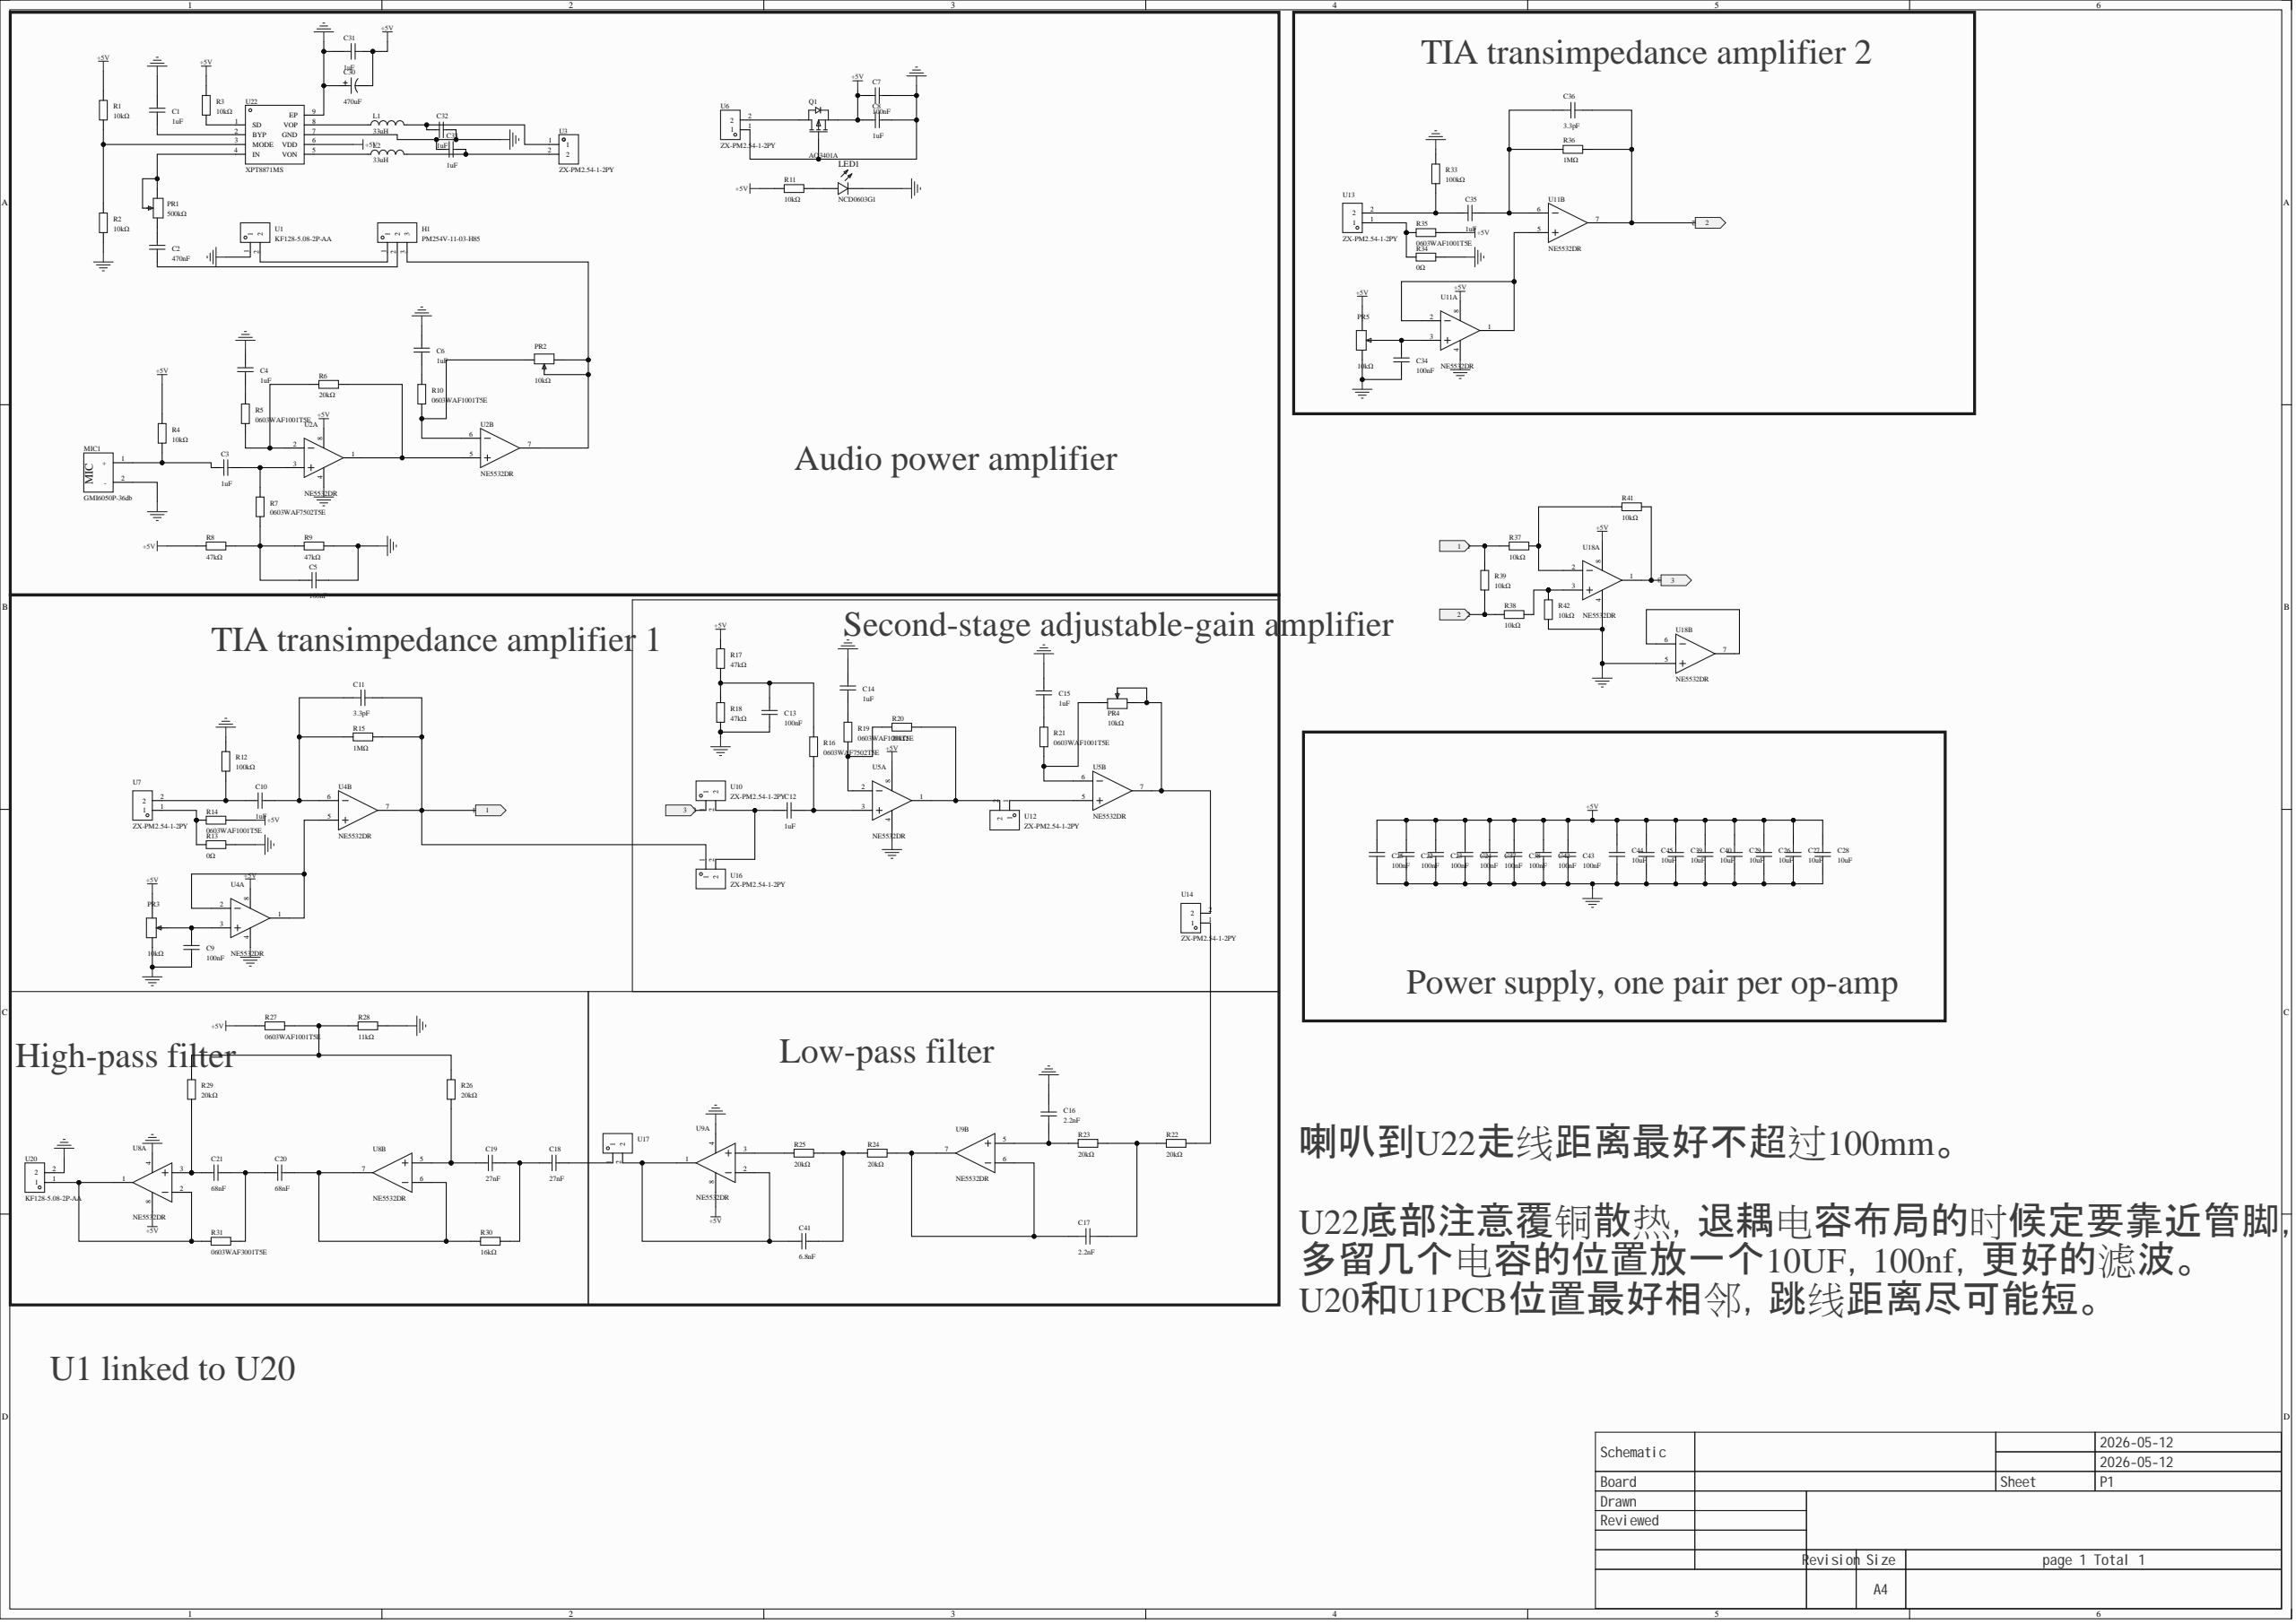Circuit board | Altium Designer | 115 parts | 65 nets
Bill of materials:
Comment,Description,Designator,Footprint,LibRef,Quantity
"1uF","Temperature coefficient: X5R; tolerance: ±10%; rated voltage: 50V; capacitance: 1uF;, Capacitance: 1uF; tolerance: ±10%; rated voltage: 50V; temperature coefficient: X5R;","C1, C3, C4, C6, C8, C10, C12, C14, C15, C31, C32, C33, C35","C0603","CL10A105KB8NNNC","13"
"470nF","Capacitance: 470nF; tolerance: ±10%; rated voltage: 16V; material (temperature coefficient): X7R;","C2","C0603","CC0603KRX7R7BB474","1"
"100nF","Capacitance: 100nF; tolerance: ±10%; rated voltage: 100V; material (temperature coefficient): X7R;","C5, C7, C9, C13, C22, C23, C24, C25, C34, C37, C38, C42, C43","C0805","CC0805KKX7R0BB104","13"
"3.3pF","Capacitance: 3.3pF; tolerance: ±0.1pF; rated voltage: 50V; material (temperature coefficient): NP0;","C11, C36","C0402","CC0402BRNPO9BN3R3","2"
"2.2nF","Temperature coefficient: X7R; capacitance: 2.2nF; tolerance: ±10%; rated voltage: 50V;","C16, C17","C0805","TCC0805X7R222K500DTS","2"
"27nF","Capacitance: 27nF; tolerance: ±10%; rated voltage: 50V; material (temperature coefficient): X7R;","C18, C19","C0603","CC0603KRX7R9BB273","2"
"68nF","Temperature coefficient: X7R; tolerance: ±10%; capacitance: 68nF; rated voltage: 50V;","C20, C21","C0603","CL10B683KB8NNNC","2"
"10uF","Capacitance: 10uF; tolerance: ±20%; rated voltage: 25V; temperature coefficient: X5R;","C26, C27, C28, C29, C39, C40, C44, C45","C0603","CL10A106MA8NRNC","8"
"470uF","Capacitance: 470uF; tolerance: ±20%; rated voltage: 35V;","C30","CAP-TH_BD10.0-P5.00-D1.0-FD","35YXJ470M10x16","1"
"6.8nF","Capacitance: 6.8nF; tolerance: ±10%; rated voltage: 50V; material (temperature coefficient): X7R;","C41","C0603","CC0603KRX7R9BB682","1"
"PM254V-11-03-H85","插孔结构:1x3P;间距:2.54mm;行距:-;圆孔/方孔:方孔;安装方式:直插;排数:单排;总孔位数:3P;额定电流:3A;插孔方向:顶部;塑高:8.5mm;触头材质:黄铜;触头镀层:-;工作温度:-40℃~+105℃;","H1","HDR-TH_3P-P2.54-V-F","PM254V-11-03-H85","1"
"33uH","Inductance: 33uH; tolerance: ±20%; rated current: 2A; DC resistance (DCR): 270mΩ;","L1, L2","IND-SMD_L7.3-W6.6","MHCI06030-330M-R8","2"
"NCD0603G1","Emitted color: emerald green;","LED1","LED0603-RD","NCD0603G1","1"
"GMI6050P-36db","","MIC1","MIC-TH_BD6.0-P1.90-D0.4-L-FD_GMI6050P-2CXXDB","GMI6050P-36db","1"
"500kΩ","Resistance: 500kΩ; tolerance: ±10%; temperature coefficient: ±100ppm/?;","PR1","RES-ADJ-TH_3296W","3296W-1-504LF","1"
"10kΩ","Resistance: 10kΩ; tolerance: ±10%; temperature coefficient: ±100ppm/?;","PR2, PR3, PR4, PR5","RES-ADJ-TH_3296W","3296W-1-103LF","4"
"AO3401A","","Q1","SOT-23_L2.9-W1.3-P1.90-LS2.4-BR","AO3401A_C15127","1"
"10kΩ","","R1, R2, R3, R4, R11, R37, R38, R39, R41, R42","R0603","0603WAF1002T5E","10"
"0603WAF1001T5E","","R5, R10, R14, R19, R21, R27, R35","R0603","0603WAF1001T5E","7"
"20kΩ","","R6, R20, R22, R23, R24, R25, R26, R29","R0603","0603WAF2002T5E","8"
"0603WAF7502T5E","","R7, R16","R0603","0603WAF7502T5E","2"
"47kΩ","","R8, R9, R17, R18","R0603","0603WAF4702T5E","4"
"100kΩ","","R12, R33","R0603","0603WAF1003T5E","2"
"0Ω","","R13, R34","R0603","0603WAF0000T5E","2"
"1MΩ","","R15, R36","R0603","0603WAF1004T5E","2"
"11kΩ","","R28","R0603","0603WAF1102T5E","1"
"16kΩ","","R30","R0603","0603WAF1602T5E","1"
"0603WAF3001T5E","","R31","R0603","0603WAF3001T5E","1"
"KF128-5.08-2P-AA","结构:1x2P;间距:5.08mm;颜色:绿色;安装方式:直插;排数:1;每排PIN数:2;额定电流:24A;额定电压:250V;线规 - AWG:12~22;线规 - 平方毫米:2.5;工作温度:-40℃~+105℃;","U1, U20","CONN-TH_P5.08_KF128-5.08-2P","KF128-5.08-2P-AA","2"
"NE5532DR","Op-amp type: General Purpose; amplifiers per package: 2; gain-bandwidth product (GBP): 10MHz; slew rate (SR): 9 V/us; supply voltage: ±5V ~ 15V; supply current per channel: 8mA;","U2, U4, U5, U8, U9, U11, U18","SOIC-8_L4.9-W3.9-P1.27-LS6.0-BL","NE5532DR","7"
"ZX-PM2.54-1-2PY","插孔结构:1x2P;间距:2.54mm;行距:-;圆孔/方孔:方孔;安装方式:直插;排数:单排;总孔位数:2P;额定电流:3A;额定电压:-;插孔方向:顶部;塑高:8.5mm;触头材质:黄铜;触头镀层:金;工作温度:-40℃~+105℃;","U3, U6, U7, U10, U12, U13, U14, U16, U17","HDR-TH_2P-P2.54-V-F","ZX-PM2.54-1-2PY","9"
"XPT8871MS","","U22","ESOP-8_L4.9-W3.9-P1.27-LS6.0-BL-EP","XPT8871MS","1"
Netlist (Protel format):
[
C1
C0603
1uF



]
[
C2
C0603
470nF



]
[
C3
C0603
1uF



]
[
C4
C0603
1uF



]
[
C5
C0805
100nF



]
[
C6
C0603
1uF



]
[
C7
C0805
100nF



]
[
C8
C0603
1uF



]
[
C9
C0805
100nF



]
[
C10
C0603
1uF



]
[
C11
C0402
3.3pF



]
[
C12
C0603
1uF



]
[
C13
C0805
100nF



]
[
C14
C0603
1uF



]
[
C15
C0603
1uF



]
[
C16
C0805
2.2nF



]
[
C17
C0805
2.2nF



]
[
C18
C0603
27nF



]
[
C19
C0603
27nF



]
[
C20
C0603
68nF



]
[
C21
C0603
68nF



]
[
C22
C0805
100nF



]
[
C23
C0805
100nF



]
[
C24
C0805
100nF



]
[
C25
C0805
100nF



]
[
C26
C0603
10uF



]
[
C27
C0603
10uF



]
[
C28
C0603
10uF



]
[
C29
C0603
10uF



]
[
C30
CAP-TH_BD10.0-P5.00-D1.0-FD
470uF



]
[
C31
C0603
1uF



]
[
C32
C0603
1uF



]
[
C33
C0603
1uF



]
[
C34
C0805
100nF



]
[
C35
C0603
1uF



]
[
C36
C0402
3.3pF



]
[
C37
C0805
100nF



]
[
C38
C0805
100nF



]
[
C39
C0603
10uF



]
[
C40
C0603
10uF



]
[
C41
C0603
6.8nF



]
[
C42
C0805
100nF



]
[
C43
C0805
100nF



]
[
C44
C0603
10uF



]
[
C45
C0603
10uF



]
[
H1
HDR-TH_3P-P2.54-V-F
PM254V-11-03-H85



]
[
L1
IND-SMD_L7.3-W6.6
33uH



]
[
L2
IND-SMD_L7.3-W6.6
33uH



]
[
LED1
LED0603-RD
NCD0603G1



]
[
MIC1
MIC-TH_BD6.0-P1.90-D0.4-L-FD_GMI6050P-2CXXDB
GMI6050P-36db



]
[
PR1
RES-ADJ-TH_3296W
500kΩ



]
[
PR2
RES-ADJ-TH_3296W
10kΩ



]
[
PR3
RES-ADJ-TH_3296W
10kΩ



]
[
PR4
RES-ADJ-TH_3296W
10kΩ



]
[
PR5
RES-ADJ-TH_3296W
10kΩ



]
[
Q1
SOT-23_L2.9-W1.3-P1.90-LS2.4-BR
AO3401A



]
[
R1
R0603
10kΩ



]
[
R2
R0603
10kΩ



]
[
R3
R0603
10kΩ



]
[
R4
R0603
10kΩ



]
[
R5
R0603
0603WAF1001T5E



]
[
R6
R0603
20kΩ



]
[
R7
R0603
0603WAF7502T5E



]
[
R8
R0603
47kΩ



]
[
R9
R0603
47kΩ



]
[
R10
R0603
0603WAF1001T5E



]
[
R11
R0603
10kΩ



]
[
R12
R0603
100kΩ



]
[
R13
R0603
0Ω



]
[
R14
R0603
0603WAF1001T5E



]
[
R15
R0603
1MΩ



]
[
R16
R0603
0603WAF7502T5E



]
[
R17
R0603
47kΩ



]
[
R18
R0603
47kΩ



]
[
R19
R0603
0603WAF1001T5E



]
[
R20
R0603
20kΩ



]
[
R21
R0603
0603WAF1001T5E



]
[
R22
R0603
20kΩ



]
[
R23
R0603
20kΩ



]
[
R24
R0603
20kΩ



]
[
R25
R0603
20kΩ



]
[
R26
R0603
20kΩ



]
[
R27
R0603
0603WAF1001T5E



]
[
R28
R0603
11kΩ



]
[
R29
R0603
20kΩ



]
[
R30
R0603
16kΩ



]
[
R31
R0603
0603WAF3001T5E



]
[
R33
R0603
100kΩ



]
[
R34
R0603
0Ω



]
[
R35
R0603
0603WAF1001T5E



]
[
R36
R0603
1MΩ



]
[
R37
R0603
10kΩ



]
[
R38
R0603
10kΩ



]
[
R39
R0603
10kΩ



]
[
R41
R0603
10kΩ



]
[
R42
R0603
10kΩ



]
[
U1
CONN-TH_P5.08_KF128-5.08-2P
KF128-5.08-2P-AA



]
[
U2
SOIC-8_L4.9-W3.9-P1.27-LS6.0-BL
NE5532DR



]
[
U3
HDR-TH_2P-P2.54-V-F
ZX-PM2.54-1-2PY



]
[
U4
SOIC-8_L4.9-W3.9-P1.27-LS6.0-BL
NE5532DR



]
[
U5
SOIC-8_L4.9-W3.9-P1.27-LS6.0-BL
NE5532DR



]
[
U6
HDR-TH_2P-P2.54-V-F
ZX-PM2.54-1-2PY



]
[
U7
HDR-TH_2P-P2.54-V-F
ZX-PM2.54-1-2PY



]
[
U8
SOIC-8_L4.9-W3.9-P1.27-LS6.0-BL
NE5532DR



]
[
U9
SOIC-8_L4.9-W3.9-P1.27-LS6.0-BL
NE5532DR



]
[
U10
HDR-TH_2P-P2.54-V-F
ZX-PM2.54-1-2PY



]
[
U11
SOIC-8_L4.9-W3.9-P1.27-LS6.0-BL
NE5532DR



]
[
U12
HDR-TH_2P-P2.54-V-F
ZX-PM2.54-1-2PY



]
[
U13
HDR-TH_2P-P2.54-V-F
ZX-PM2.54-1-2PY



]
[
U14
HDR-TH_2P-P2.54-V-F
ZX-PM2.54-1-2PY



]
[
U16
HDR-TH_2P-P2.54-V-F
ZX-PM2.54-1-2PY



]
[
U17
HDR-TH_2P-P2.54-V-F
ZX-PM2.54-1-2PY



]
[
U18
SOIC-8_L4.9-W3.9-P1.27-LS6.0-BL
NE5532DR



]
[
U20
CONN-TH_P5.08_KF128-5.08-2P
KF128-5.08-2P-AA



]
[
U22
ESOP-8_L4.9-W3.9-P1.27-LS6.0-BL-EP
XPT8871MS



]
(
NetU18_6
U18-6
U18-7
)
(
NetU11_1
U11-1
U11-2
U11-5
)
(
NetU5_5
U5-5
U12-1
)
(
NetU4_1
U4-1
U4-2
U4-5
)
(
NetR38_2
R38-2
R42-2
U18-3
)
(
NetR37_2
R37-2
R41-2
U18-2
)
(
NetR34_1
R34-1
R35-1
U13-1
)
(
NetR31_1
R31-1
U8-1
U8-2
U20-1
)
(
NetR26_2
R26-2
R27-1
R28-2
R29-1
)
(
NetR25_1
R25-1
U9-3
)
(
NetR22_2
R22-2
U14-1
)
(
NetR20_2
R20-2
U5-1
U12-2
)
(
NetR19_1
R19-1
R20-1
U5-2
)
(
NetR13_1
R13-1
R14-1
U7-1
)
(
NetR6_1
R6-1
U2-1
U2-5
)
(
NetR5_1
R5-1
R6-2
U2-2
)
(
NetR3_1
R3-1
U22-1
)
(
NetR1_1
R1-1
R2-2
U22-3
)
(
NetQ1_3
Q1-3
U6-2
)
(
NetPR4_3
PR4-3
R21-1
U5-6
)
(
NetPR4_1
PR4-1
PR4-2
U5-7
U14-2
)
(
NetPR2_1
PR2-1
R10-2
U2-6
)
(
NetPR1_1
PR1-1
PR1-2
U22-4
)
(
NetLED1_2
LED1-2
R11-2
)
(
NetL2_1
L2-1
U22-5
)
(
NetL1_1
L1-1
U22-8
)
(
NetH1_3
H1-3
PR2-2
PR2-3
U2-7
)
(
NetH1_1
H1-1
U1-2
)
(
NetC41_2
C41-2
R24-1
R25-2
)
(
NetC41_1
C41-1
U9-1
U9-2
U17-2
)
(
NetC35_2
C35-2
C36-2
R36-1
U11-6
)
(
NetC35_1
C35-1
R33-1
U13-2
)
(
NetC34_2
C34-2
PR5-2
U11-3
)
(
NetC33_2
C33-2
L2-2
U3-2
)
(
NetC32_1
C32-1
L1-2
U3-1
)
(
NetC21_1
C21-1
R29-2
U8-3
)
(
NetC20_2
C20-2
R30-1
U8-6
U8-7
)
(
NetC20_1
C20-1
C21-2
R31-2
)
(
NetC19_1
C19-1
R26-1
U8-5
)
(
NetC18_2
C18-2
U17-1
)
(
NetC18_1
C18-1
C19-2
R30-2
)
(
NetC17_2
C17-2
R24-2
U9-6
U9-7
)
(
NetC17_1
C17-1
R22-1
R23-2
)
(
NetC16_2
C16-2
R23-1
U9-5
)
(
NetC15_1
C15-1
R21-2
)
(
NetC14_1
C14-1
R19-2
)
(
NetC13_2
C13-2
R16-2
R17-1
R18-2
)
(
NetC12_2
C12-2
R16-1
U5-3
)
(
NetC12_1
C12-1
U10-2
U16-2
)
(
NetC10_2
C10-2
C11-2
R15-1
U4-6
)
(
NetC10_1
C10-1
R12-1
U7-2
)
(
NetC9_2
C9-2
PR3-2
U4-3
)
(
NetC6_1
C6-1
R10-1
)
(
NetC5_1
C5-1
R7-1
R8-1
R9-2
)
(
NetC4_1
C4-1
R5-2
)
(
NetC3_2
C3-2
R7-2
U2-3
)
(
NetC3_1
C3-1
MIC1-1
R4-1
)
(
NetC2_2
C2-2
PR1-3
)
(
NetC2_1
C2-1
H1-2
)
(
NetC1_1
C1-1
U22-2
)
(
GND
C1-2
C4-2
C5-2
C6-2
C7-2
C8-2
C9-1
C13-1
C14-2
C15-2
C16-1
C22-1
C23-1
C24-1
C25-1
C26-1
C27-1
C28-1
C29-1
C30-1
C31-1
C32-2
C33-1
C34-1
C37-1
C38-1
C39-1
C40-1
C42-1
C43-1
C44-1
C45-1
LED1-1
MIC1-2
PR3-1
PR5-1
Q1-1
R2-1
R9-1
R12-2
R13-2
R18-1
R28-1
R33-2
R34-2
R42-1
U1-1
U2-4
U4-4
U5-4
U6-1
U8-4
U9-4
U11-4
U18-4
U18-5
U20-2
U22-7
U22-9
)
(
+5V
C7-1
C8-1
C22-2
C23-2
C24-2
C25-2
C26-2
C27-2
C28-2
C29-2
C30-2
C31-2
C37-2
C38-2
C39-2
C40-2
C42-2
C43-2
C44-2
C45-2
PR3-3
PR5-3
Q1-2
R1-2
R3-2
R4-2
R8-2
R11-1
R14-2
R17-2
R27-2
R35-2
U2-8
U4-8
U5-8
U8-8
U9-8
U11-8
U18-8
U22-6
)
(
3
R41-1
U10-1
U18-1
)
(
2
C36-1
R36-2
R38-1
R39-1
U11-7
)
(
1
C11-1
R15-2
R37-1
R39-2
U4-7
U16-1
)